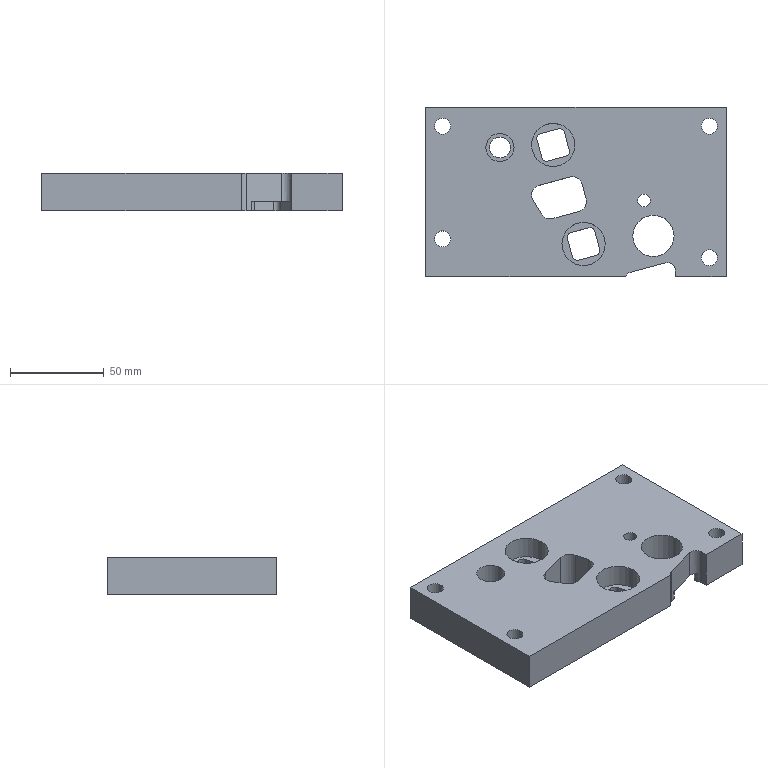Part | NX | features solid 2 | 1 solid | 67 faces | box 160 x 90 x 20 mm | volume 239062 mm3 | cylinder 34 | plane 33 | commonest cylinder face diameters 5.15 x8 6 x4 8.5 x4 11 x4 14 x4 4 x2